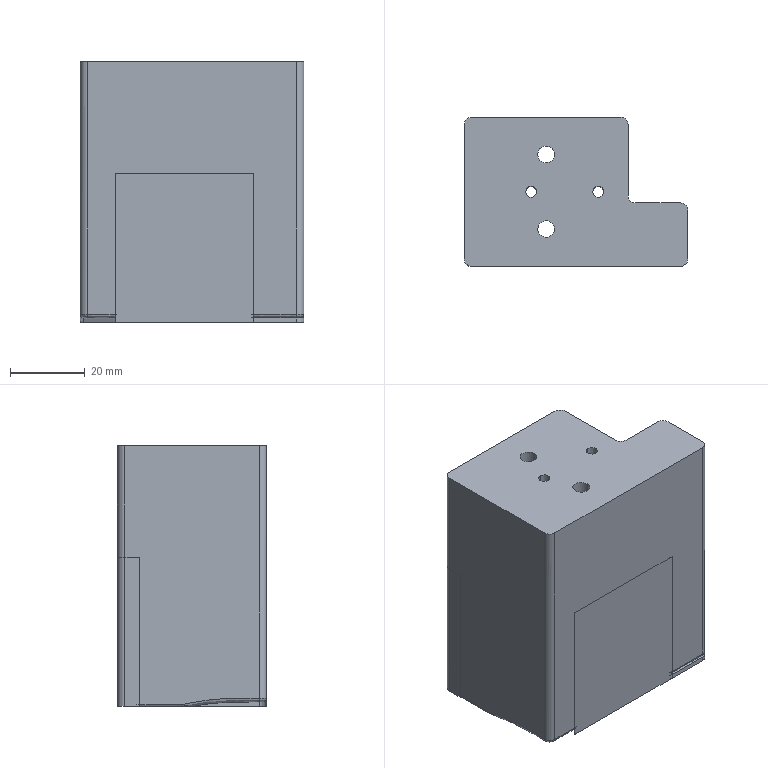NC program | NX | posted with a generic post | part box 60.004 x 40.015 x 70 mm
Whole program:
N10 G17 G21 G94 G90
(FLOOR_WALL_COPY , TOOL : D63)
N12 T01 M6
N14 G54
N16 G17 G0 G90 X69.5 Y-29.997 B0. C0. S6500 M3
N18 G43 Z30. H1
N20 Z7.179
N22 G94 G1 Z4.179 F1250.
N24 X66.5
N26 X-66.5
N28 Y-25.531
N30 Y-12.597
N32 X66.5
N34 Y4.804
N36 X-66.5
N38 X-69.5
N40 Z7.179
N42 G0 Z30.
N44 X69.5 Y-29.997
N46 Z6.343
N48 G1 Z3.343
N50 X66.5
N52 X-66.5
N54 Y-12.597
N56 X66.5
N58 Y4.804
N60 X-66.5
N62 X-69.5
N64 Z6.343
N66 G0 Z30.
N68 X69.5 Y-29.997
N70 Z5.507
N72 G1 Z2.507
N74 X66.5
N76 X-66.5
N78 Y-12.597
N80 X66.5
N82 Y4.804
N84 X-66.5
N86 X-69.5
N88 Z5.507
N90 G0 Z30.
N92 X69.5 Y-29.997
N94 Z4.672
N96 G1 Z1.672
N98 X66.5
N100 X-66.5
N102 Y-12.597
N104 X66.5
N106 Y4.804
N108 X-66.5
N110 X-69.5
N112 Z4.672
N114 G0 Z30.
N116 X69.5 Y-29.997
N118 Z3.836
N120 G1 Z0.836
N122 X66.5
N124 X-66.5
N126 Y-12.597
N128 X66.5
N130 Y4.804
N132 X-66.5
N134 X-69.5
N136 Z3.836
N138 G0 Z30.
N140 X69.5 Y-29.997
N142 Z3.
N144 G1 Z0.
N146 X66.5
N148 X-66.5
N150 Y-12.597
N152 X66.5
N154 Y4.804
N156 X-66.5
N158 X-69.5
N160 Z3.
N162 G0 Z30.
N164 M5
(ZLEVEL_PROFILE_COPY_COPY_2 , TOOL : D6R0.5)
N166 T08 M6
N168 G54
N170 G17 G0 G90 X-39.271 Y31.633 B0. C0. S9500 M3
N172 G43 Z30. H8
N174 Z1.495
N176 G94 G1 Z-0.005 F1000.
N178 X-38.821 Y30.859
N180 G3 X-38.3 Y30.56 R0.6
N182 G1 X-35.602 Y30.569 F3000.
N184 X-35. Y30.658
N186 X32.8
N188 G3 X33.638 Y30.635 R2.218
N190 X34.785 Y30.792 R5.772
N192 G1 X35.889 Y30.637
N194 X36.022 Y30.598
N196 X36.086 Y30.572
N198 X36.094
N200 X36.101 Y30.618 Z-0.01
N202 X36.018 Y30.638
N204 G3 X34.785 Y30.826 R4.354
N206 G1 X33.635 Y30.677
N208 G2 X32.8 Y30.723 R1.702
N210 G1 X-35.
N212 X-35.602 Y30.641
N214 X-35.947 Y30.617
N216 X-38.3 Y30.602
N218 Y30.628 Z-0.014
N220 Y30.641 Z-0.018
N222 G3 X-35. Y30.798 R17.351
N224 G1 X32.8
N226 G3 X33.629 Y30.743 R1.604
N228 G1 X34.493 Y30.845
N230 G2 X35.962 Y30.714 R3.573
N232 G1 X36.101 Y30.67
N234 X36.1 Y30.732 Z-0.027
N236 X35.897 Y30.788
N238 G3 X34.685 Y30.936 R2.892
N240 G1 X33.622 Y30.822
N242 X32.8 Y30.868
N244 X-35.
N246 G2 X-38.3 Y30.688 R16.479
N248 G1 Y30.736 Z-0.033
N250 Y30.745 Z-0.039
N252 G3 X-35. Y30.937 R15.652
N254 G1 X32.8
N256 X33.614 Y30.918
N258 X33.78 Y30.936
N260 X35.062 Y30.988
N262 G2 X35.897 Y30.849 R2.083
N264 G1 X36.1 Y30.808
N266 Y30.866 Z-0.045
N268 Y30.896 Z-0.052
N270 X35.838 Y30.935
N272 X35.13 Y31.044
N274 X33.624 Y30.981
N276 X32.8 Y31.008
N278 X-35.
N280 G2 X-38.3 Y30.812 R15.552
N282 G1 Y30.866 Z-0.06
N284 Y30.89 Z-0.068
N286 G3 X-35. Y31.078 R15.987
N288 G1 X32.8
N290 X33.639 Y31.043
N292 X35.13 Y31.106
N294 X35.743 Y31.02
N296 X35.804 Y31.003
N298 X36.076 Y30.973
N300 Y31.02 Z-0.077
N302 X36.077 Y31.041 Z-0.085
N304 X35.82 Y31.061
N306 X35.778 Y31.075
N308 G3 X33.657 Y31.114 R7.673
N310 G1 X32.8 Y31.148
N312 X-35.
N314 G2 X-38.3 Y30.968 R16.512
N316 G1 Y31.013 Z-0.096
N318 Y31.047 Z-0.107
N320 G3 X-35. Y31.223 R18.029
N322 G1 X32.8
N324 X33.678 Y31.2
N326 G2 X35.746 Y31.159 R7.532
N328 G1 X36.077 Y31.123
N330 X36.078 Y31.187 Z-0.119
N332 Y31.22 Z-0.132
N334 X35.767 Y31.235
N336 X35.701 Y31.25
N338 G3 X35.13 Y31.33 R2.098
N340 G1 X33.699 Y31.294
N342 X32.8 Y31.302
N344 X-35.
N346 G2 X-38.3 Y31.142 R22.279
N348 G1 Y31.207 Z-0.147
N350 Y31.252 Z-0.162
N352 G3 X-35. Y31.384 R27.541
N354 G1 X32.8
N356 X33.706 Y31.367
N358 G2 X35.662 Y31.34 R9.516
N360 G1 X36.1 Y31.318
N362 Y31.365 Z-0.178
N364 Y31.408 Z-0.195
N366 X35.636 Y31.427
N368 X35.475 Y31.461
N370 X33.714 Y31.449
N372 X32.8 Y31.468
N374 X-35.
N376 G2 X-38.3 Y31.342 R25.762
N378 G1 Y31.386 Z-0.214
N380 Y31.43 Z-0.232
N382 G3 X-35. Y31.552 R26.651
N384 G1 X32.8
N386 X33.723 Y31.537
N388 G2 X35.612 Y31.51 R9.631
N390 G1 X35.638 Y31.504
N392 X36.1 Y31.497
N394 Y31.541 Z-0.253
N396 Y31.583 Z-0.273
N398 X35.646 Y31.587
N400 X35.585 Y31.599
N402 X35.13 Y31.659
N404 X33.732 Y31.633
N406 X32.8 Y31.636
N408 X-35.
N410 G2 X-38.3 Y31.526 R31.082
N412 G1 Y31.579 Z-0.295
N414 Y31.63 Z-0.318
N416 G3 X-35. Y31.72 R34.974
N418 G1 X32.8
N420 X33.736 Y31.708
N422 G2 X35.565 Y31.684 R8.833
N424 G1 X35.625 Y31.672
N426 X36.1 Y31.669
N428 Y31.715 Z-0.342
N430 Y31.754 Z-0.366
N432 X35.632 Y31.757
N434 X35.548 Y31.771
N436 G3 X33.741 Y31.788 R8.723
N438 G1 X32.8 Y31.802
N440 X-35.
N442 G2 X-38.3 Y31.705 R31.855
N444 G1 Y31.757 Z-0.392
N446 Y31.786 Z-0.417
N448 G3 X-35. Y31.883 R31.669
N450 G1 X32.8
N452 X33.746 Y31.874
N454 G2 X35.527 Y31.854 R10.532
N456 G1 X35.64 Y31.839
N458 X36.1 Y31.838
N460 Y31.882 Z-0.445
N462 Y31.919 Z-0.473
N464 X35.504 Y31.936
N466 X35.13 Y31.979
N468 X33.75 Y31.961
N470 G2 X32.8 Y31.963 R56.426
N472 G1 X-35.
N474 G2 X-38.3 Y31.872 R35.01
N476 G1 Y31.92 Z-0.502
N478 Y31.963 Z-0.531
N480 G3 X-35. Y32.04 R43.86
N482 G1 X32.8
N484 G3 X33.753 Y32.035 R59.868
N486 G2 X35.481 Y32.018 R11.944
N488 G1 X36.1 Y31.999
N490 Y32.042 Z-0.562
N492 Y32.075 Z-0.593
N494 X35.461 Y32.093
N496 X35.13 Y32.128
N498 X33.756 Y32.112
N500 G2 X32.8 Y32.116 R59.942
N502 G1 X-35.
N504 G2 X-38.3 Y32.052 R53.65
N506 G1 Y32.086 Z-0.625
N508 Y32.122 Z-0.657
N510 G3 X-35. Y32.19 R48.77
N512 G1 X32.8
N514 G3 X33.759 Y32.185 R9.711
N516 G1 X35.13 Y32.199
N518 X35.442 Y32.169
N520 X36.1 Y32.154
N522 Y32.192 Z-0.691
N524 Y32.223 Z-0.725
N526 X35.422 Y32.24
N528 X35.13 Y32.269
N530 X33.762 Y32.256
N532 G2 X32.8 Y32.261 R8.87
N534 G1 X-35.
N536 G2 X-38.3 Y32.191 R44.855
N538 G1 Y32.227 Z-0.761
N540 Y32.262 Z-0.796
N542 G3 X-35. Y32.329 R47.111
N544 G1 X32.8
N546 G3 X33.776 Y32.328 R11.732
N548 G1 X35.13 Y32.338
N550 X35.4 Y32.313
N552 X35.475 Y32.302
N554 X36.1 Y32.295
N556 Y32.331 Z-0.833
N558 Y32.36 Z-0.869
N560 X35.475 Y32.364
N562 X35.386 Y32.377
N564 X35.13 Y32.4
N566 X33.85 Y32.391
N568 G2 X32.8 Y32.395 R10.452
N570 G1 X-35.
N572 G2 X-38.3 Y32.334 R54.066
N574 G1 Y32.369 Z-0.908
N576 Y32.406 Z-0.946
N578 G3 X-35. Y32.458 R60.994
N580 G1 X32.8
N582 G3 X33.928 Y32.457 R12.222
N584 G1 X35.13 Y32.464
N586 X35.387 Y32.44
N588 X35.475 Y32.426
N590 X36.1 Y32.423
N592 Y32.459 Z-0.985
N594 Y32.488 Z-1.025
N596 X35.475 Y32.49
N598 X35.387 Y32.5
N600 X35.13 Y32.522
N602 X34.008 Y32.516
N604 G2 X32.8 Y32.518 R17.829
N606 G1 X-35.
N608 G2 X-38.3 Y32.46 R54.632
N610 G1 Y32.489 Z-1.065
N612 Y32.515 Z-1.106
N614 G3 X-35. Y32.575 R51.838
N616 G1 X32.8
N618 X32.834 Y32.574
N620 G3 X34.09 Y32.577 R13.678
N622 G1 X35.215 Y32.572
N624 G3 X36.1 Y32.542 R6.159
N626 G1 Y32.574 Z-1.148
N628 Y32.597 Z-1.189
N630 G2 X35.216 Y32.625 R6.651
N632 G1 X35.13 Y32.631
N634 X34.19 Y32.629
N636 G2 X32.8 Y32.629 R20.855
N638 G1 X-35.
N640 G2 X-38.3 Y32.57 R53.013
N642 G1 Y32.601 Z-1.232
N644 Y32.627 Z-1.275
N646 G3 X-35. Y32.679 R67.937
N648 G1 X32.8
N650 G3 X34.326 Y32.682 R29.126
N652 G1 X35.086 Y32.685
N654 X35.231 Y32.678
N656 G3 X36.1 Y32.652 R7.22
N658 G1 Y32.676 Z-1.319
N660 Y32.696 Z-1.363
N662 X35.475 Y32.698
N664 X35.097 Y32.732
N666 X35.081 Y32.73
N668 X34.758 Y32.732
N670 G2 X33.75 Y32.723 R58.276
N672 X32.8 Y32.727 R7.956
N674 G1 X-35.
N676 X-35.257 Y32.71
N678 X-36.637 Y32.679
N680 X-36.982 Y32.678
N682 X-38.3
N684 Y32.699 Z-1.408
N686 Y32.716 Z-1.453
N688 G3 X-35.346 Y32.75 R70.002
N690 X-35. Y32.77 R6.897
N692 G1 X32.8
N694 G3 X33.75 Y32.767 R7.265
N696 X34.984 Y32.774 R66.563
N698 G1 X35.076
N700 X35.081 Y32.772
N702 X35.13 Y32.774
N704 X35.475 Y32.739
N706 X36.1 Y32.737
N708 Y32.766 Z-1.498
N710 Y32.779 Z-1.544
N712 G2 X35.13 Y32.812 R7.451
N714 G1 X33.75 Y32.806
N716 X33.567 Y32.801
N718 G2 X32.8 Y32.81 R9.097
N720 G1 X-35.
N722 G2 X-38.3 Y32.756 R53.601
N724 G1 Y32.777 Z-1.591
N726 Y32.795 Z-1.637
N728 G3 X-35. Y32.846 R63.067
N730 G1 X32.8
N732 G3 X33.04 Y32.84 R4.138
N734 G1 X35.13 Y32.848
N736 G3 X36.1 Y32.822 R9.315
N738 G1 Y32.841 Z-1.684
N740 Y32.854 Z-1.732
N742 G2 X34.979 Y32.882 R14.001
N744 X33.059 Y32.87 R208.89
N746 G1 X32.8 Y32.879
N748 X-35.
N750 G2 X-38.3 Y32.834 R71.019
N752 G1 Y32.847 Z-1.779
N754 Y32.861 Z-1.827
N756 G3 X-35. Y32.908 R78.959
N758 G1 X32.8
N760 G3 X33.577 Y32.901 R10.862
N762 G1 X33.75 Y32.905
N764 X35.087 Y32.909
N766 X35.13 Y32.906
N768 G3 X36.1 Y32.885 R10.979
N770 G1 Y32.902 Z-1.876
N772 Y32.915 Z-1.924
N774 G2 X34.99 Y32.934 R19.534
N776 X33.059 Y32.927 R978.128
N778 G1 X32.8 Y32.933
N780 X-35.
N782 G2 X-38.3 Y32.889 R102.631
N784 G1 Y32.904 Z-1.973
N786 X-38.301 Y32.916 Z-2.022
N788 G3 X-35. Y32.954 R128.005
N790 G1 X32.8
N792 X33.059 Y32.951
N794 X34.98 Y32.956
N796 G3 X36.1 Y32.938 R20.185
N798 G1 X36.101 Y32.95 Z-2.071
N800 Y32.958 Z-2.12
N802 G2 X34.99 Y32.974 R20.02
N804 G1 X33.059 Y32.968
N806 X32.8 Y32.971
N808 X-35.
N810 G2 X-38.301 Y32.94 R191.718
N812 G1 Y32.948 Z-2.168
N814 Y32.96 Z-2.215
N816 X-35.602 Y32.973
N818 X-35. Y32.984
N820 X32.8
N822 G2 X36.101 Y32.97 R480.36
N824 G1 Y32.979 Z-2.31
N826 X35.245 Y32.982
N828 X35.077 Y32.989
N830 X33.059 Y32.986
N832 X32.8 Y32.993
N834 X-35.
N836 X-35.257 Y32.988
N838 X-38.301 Y32.975
N840 Y32.981 Z-2.358
N842 X-38.3 Y32.99 Z-2.405
N844 X-35. Y32.998
N846 X32.8
N848 X33.059 Y32.994
N850 X35.077 Y32.997
N852 X35.246 Y32.987
N854 X36.101 Y32.985
N856 X36.1 Y32.988 Z-2.5
N858 X35.246 Y32.987
N860 X35.077 Y32.998
N862 X-38.3 Y32.997
N864 G2 X-38.819 Y33.297 R0.6
N866 G1 X-39.273 Y34.083
N868 Z-1.
N870 G0 Z30.
N872 X37.084 Y-31.601
N874 Z1.495
N876 G1 Z-0.005 F1000.
N878 X36.625 Y-30.836
N880 G3 X36.1 Y-30.545 R0.6
N882 G1 X33.389 Y-30.591 F3000.
N884 X32.8 Y-30.658
N886 X-35.
N888 X-35.257 Y-30.616
N890 X-38.3 Y-30.556
N892 Y-30.586 Z-0.008
N894 Y-30.598 Z-0.01
N896 X-36.637 Y-30.608
N898 X-36.292 Y-30.616
N900 G2 X-35. Y-30.723 R9.19
N902 G1 X32.8
N904 X33.404 Y-30.633
N906 X36.1 Y-30.607
N908 Y-30.645 Z-0.014
N910 Y-30.661 Z-0.018
N912 X33.404 Y-30.7
N914 X32.8 Y-30.798
N916 X-35.
N918 G3 X-38.3 Y-30.634 R21.565
N920 G1 Y-30.661 Z-0.022
N922 Y-30.677 Z-0.027
N924 G2 X-35. Y-30.868 R20.632
N926 G1 X32.8
N928 X33.404 Y-30.782
N930 X36.1 Y-30.727
N932 Y-30.796 Z-0.033
N934 Y-30.806 Z-0.039
N936 X33.404 Y-30.881
N938 X32.8 Y-30.937
N940 X-35.
N942 G3 X-38.3 Y-30.73 R20.154
N944 G1 Y-30.767 Z-0.045
N946 Y-30.792 Z-0.052
N948 G2 X-35. Y-31.008 R21.096
N950 G1 X32.8
N952 X33.059 Y-30.981
N954 X36.1 Y-30.901
N956 Y-30.951 Z-0.06
N958 Y-30.976 Z-0.068
N960 X33.059 Y-31.042
N962 X32.8 Y-31.078
N964 X-35.
N966 G3 X-38.3 Y-30.864 R22.658
N968 G1 Y-30.907 Z-0.077
N970 Y-30.944 Z-0.085
N972 G2 X-35. Y-31.148 R21.76
N974 G1 X32.8
N976 X33.059 Y-31.112
N978 X36.1 Y-31.043
N980 Y-31.101 Z-0.096
N982 Y-31.124 Z-0.107
N984 X32.8 Y-31.223
N986 X-35.
N988 G3 X-38.3 Y-31.03 R22.476
N990 G1 Y-31.096 Z-0.119
N992 Y-31.132 Z-0.132
N994 G2 X-35. Y-31.302 R26.08
N996 G1 X32.8
N998 X36.1 Y-31.221
N1000 Y-31.274 Z-0.147
N1002 Y-31.318 Z-0.162
N1004 X32.8 Y-31.384
N1006 X-35.
N1008 G3 X-38.3 Y-31.25 R28.866
N1010 G1 Y-31.3 Z-0.178
N1012 Y-31.342 Z-0.195
N1014 G2 X-35. Y-31.468 R25.762
N1016 G1 X32.8
N1018 X36.1 Y-31.409
N1020 Y-31.452 Z-0.214
N1022 Y-31.497 Z-0.232
N1024 X32.8 Y-31.552
N1026 X-35.
N1028 G3 X-38.3 Y-31.43 R26.651
N1030 G1 Y-31.478 Z-0.253
N1032 Y-31.526 Z-0.273
N1034 G2 X-35. Y-31.636 R31.082
N1036 G1 X32.8
N1038 X36.1 Y-31.583
N1040 Y-31.629 Z-0.295
N1042 Y-31.669 Z-0.318
N1044 X33.059 Y-31.706
N1046 X32.8 Y-31.72
N1048 X-35.
N1050 G3 X-38.3 Y-31.63 R34.974
N1052 G1 Y-31.674 Z-0.342
N1054 Y-31.705 Z-0.366
N1056 G2 X-35. Y-31.802 R31.855
N1058 G1 X32.8
N1060 X36.1 Y-31.754
N1062 Y-31.8 Z-0.392
N1064 Y-31.838 Z-0.417
N1066 X33.059 Y-31.871
N1068 X32.8 Y-31.883
N1070 X-35.
N1072 G3 X-38.3 Y-31.786 R31.669
N1074 G1 Y-31.836 Z-0.445
N1076 Y-31.872 Z-0.473
N1078 G2 X-35. Y-31.963 R35.01
N1080 G1 X32.8
N1082 X33.059 Y-31.953
N1084 X36.1 Y-31.919
N1086 Y-31.963 Z-0.502
N1088 Y-31.999 Z-0.531
N1090 X33.059 Y-32.029
N1092 X32.8 Y-32.04
N1094 X-35.
N1096 G3 X-38.3 Y-31.963 R43.86
N1098 G1 Y-32.007 Z-0.562
N1100 Y-32.052 Z-0.593
N1102 G2 X-35. Y-32.116 R53.65
N1104 G1 X32.8
N1106 X33.059 Y-32.106
N1108 X36.1 Y-32.075
N1110 Y-32.118 Z-0.625
N1112 Y-32.154 Z-0.657
N1114 X33.059 Y-32.18
N1116 X32.8 Y-32.19
N1118 X-35.
N1120 G3 X-38.3 Y-32.122 R48.77
N1122 G1 Y-32.157 Z-0.691
N1124 Y-32.191 Z-0.725
N1126 G2 X-35. Y-32.261 R44.855
N1128 G1 X32.8
N1130 X33.059 Y-32.25
N1132 X36.1 Y-32.223
N1134 Y-32.262 Z-0.761
N1136 Y-32.295 Z-0.796
N1138 X33.059 Y-32.323
N1140 X32.8 Y-32.329
N1142 X-35.
N1144 G3 X-38.3 Y-32.262 R47.111
N1146 G1 Y-32.299 Z-0.833
N1148 Y-32.334 Z-0.869
N1150 G2 X-35. Y-32.395 R54.066
N1152 G1 X32.8
N1154 X33.059 Y-32.384
N1156 X35.82 Y-32.361
N1158 X36.1 Y-32.36
N1160 Y-32.396 Z-0.908
N1162 Y-32.423 Z-0.946
N1164 X35.82 Y-32.424
N1166 X33.059 Y-32.448
N1168 X32.8 Y-32.458
N1170 X-35.
N1172 G3 X-38.3 Y-32.406 R60.994
N1174 G1 Y-32.433 Z-0.985
N1176 Y-32.46 Z-1.025
N1178 G2 X-35. Y-32.518 R54.632
N1180 G1 X32.8
N1182 X33.059 Y-32.51
N1184 X35.82 Y-32.489
N1186 X36.1 Y-32.488
N1188 Y-32.519 Z-1.065
N1190 Y-32.542 Z-1.106
N1192 G3 X32.8 Y-32.575 R110.616
N1194 G1 X-35.
N1196 G3 X-38.3 Y-32.515 R51.838
N1198 G1 Y-32.544 Z-1.148
N1200 Y-32.57 Z-1.189
N1202 G2 X-35. Y-32.629 R53.013
N1204 G1 X32.8
N1206 G2 X36.1 Y-32.597 R117.59
N1208 G1 Y-32.628 Z-1.232
N1210 Y-32.653 Z-1.275
N1212 X35.82 Y-32.654
N1214 X33.059 Y-32.673
N1216 X32.8 Y-32.679
N1218 X-35.
N1220 G3 X-38.3 Y-32.627 R67.937
N1222 G1 Y-32.652 Z-1.319
N1224 Y-32.678 Z-1.363
N1226 X-36.982
N1228 X-36.637 Y-32.679
N1230 X-35.257 Y-32.71
N1232 X-35. Y-32.727
N1234 X32.8
N1236 G2 X36.1 Y-32.696 R92.346
N1238 G1 Y-32.723 Z-1.408
N1240 Y-32.737 Z-1.453
N1242 X34.44 Y-32.741
N1244 X33.059 Y-32.758
N1246 X32.8 Y-32.77
N1248 X-35.
N1250 G3 X-35.348 Y-32.75 R6.932
N1252 X-38.3 Y-32.716 R69.893
N1254 G1 Y-32.738 Z-1.498
N1256 Y-32.756 Z-1.544
N1258 G2 X-35. Y-32.81 R53.601
N1260 G1 X32.8
N1262 G2 X36.1 Y-32.779 R121.031
N1264 G1 Y-32.803 Z-1.591
N1266 Y-32.821 Z-1.637
N1268 G3 X32.8 Y-32.846 R190.89
N1270 G1 X-35.
N1272 G3 X-38.3 Y-32.795 R62.664
N1274 G1 Y-32.815 Z-1.684
N1276 Y-32.834 Z-1.732
N1278 G2 X-35. Y-32.879 R71.69
N1280 G1 X32.8
N1282 G2 X36.1 Y-32.854 R155.556
N1284 G1 Y-32.871 Z-1.779
N1286 Y-32.884 Z-1.827
N1288 G3 X32.8 Y-32.908 R176.632
N1290 G1 X-35.
N1292 G3 X-38.3 Y-32.863 R74.052
N1294 G1 Y-32.88 Z-1.876
N1296 Y-32.893 Z-1.924
N1298 G2 X-35. Y-32.933 R74.955
N1300 G1 X32.8
N1302 X33.059 Y-32.928
N1304 X36.101 Y-32.914
N1306 Y-32.925 Z-1.973
N1308 Y-32.938 Z-2.022
N1310 X33.059 Y-32.951
N1312 X32.8 Y-32.954
N1314 X-35.
N1316 G3 X-38.301 Y-32.921 R90.571
N1318 G1 Y-32.931 Z-2.071
N1320 Y-32.945 Z-2.12
N1322 G2 X-35. Y-32.971 R119.078
N1324 G1 X32.8
N1326 X33.404 Y-32.965
N1328 X36.101 Y-32.957
N1330 Y-32.964 Z-2.168
N1332 Y-32.97 Z-2.215
N1334 X32.8 Y-32.984
N1336 X-35.
N1338 G3 X-38.301 Y-32.963 R132.051
N1340 G1 Y-32.973 Z-2.263
N1342 Y-32.977 Z-2.31
N1344 X-38.017
N1346 X-35.257 Y-32.986
N1348 X-35. Y-32.993
N1350 X32.8
N1352 X33.059 Y-32.987
N1354 X36.1 Y-32.978
N1356 Y-32.984 Z-2.405
N1358 X33.404 Y-32.99
N1360 X32.8 Y-32.998
N1362 X-35.
N1364 X-35.257 Y-32.994
N1366 X-38.3 Y-32.991
N1368 X-38.298 Y-32.999 Z-2.5
N1370 X32.714
N1372 G2 X36.1 Y-32.986 R483.909
N1374 X36.619 Y-33.286 R0.6
N1376 G1 X37.074 Y-34.073
N1378 Z-1.
N1380 G0 Z30.
N1382 M5
N1384 M2